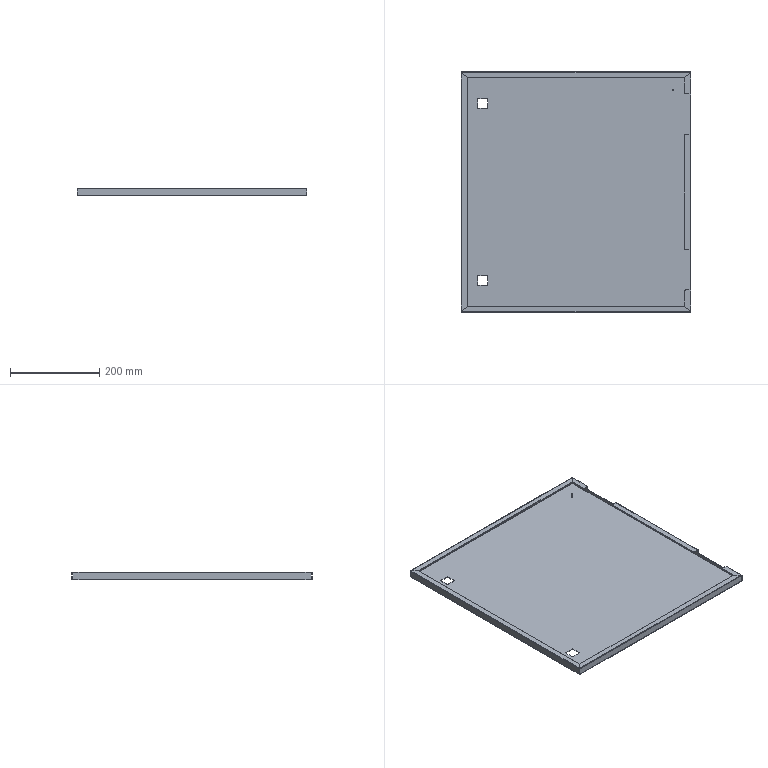Part | STEP file | Door panel | 1 solid | 129 faces | box 515 x 539 x 17 mm | volume 394918 mm3 | plane 95 | cylinder 26 | spline 8 | commonest cylinder face diameters 0.02 x10 2.42 x10 2 x4 3 x2